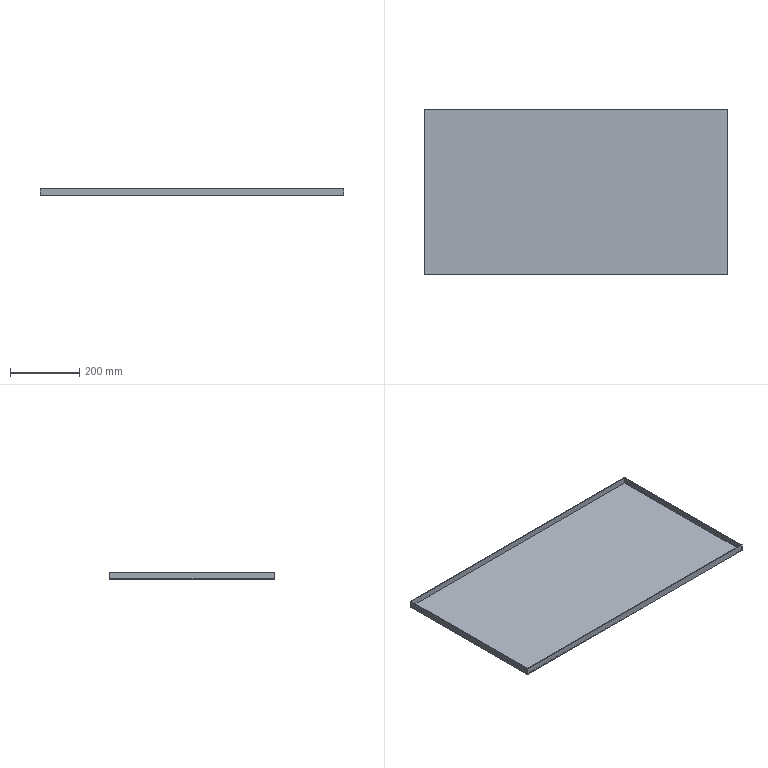Part | STEP file | Sealing plate | 1 solid | 11 faces | box 880 x 480 x 20 mm | volume 942432 mm3 | plane 11
STEP:
#1=CARTESIAN_POINT('',(0.,0.,0.));
#2=DIRECTION('',(0.,0.,1.));
#3=DIRECTION('',(1.,0.,0.));
#4=AXIS2_PLACEMENT_3D('',#1,#2,#3);
#5=CARTESIAN_POINT('',(-440.,-240.,0.));
#6=VERTEX_POINT('',#5);
#7=CARTESIAN_POINT('',(440.,-240.,0.));
#8=VERTEX_POINT('',#7);
#9=CARTESIAN_POINT('',(0.,-240.,0.));
#10=DIRECTION('',(1.,0.,0.));
#11=VECTOR('',#10,1.);
#12=LINE('',#9,#11);
#13=CARTESIAN_POINT('',(0.,0.,0.));
#14=DIRECTION('',(0.,0.,1.));
#15=DIRECTION('',(1.,0.,0.));
#16=AXIS2_PLACEMENT_3D('',#13,#14,#15);
#17=PLANE('',#16);
#18=CARTESIAN_POINT('',(0.,-240.));
#19=DIRECTION('',(1.,0.));
#20=VECTOR('',#19,1.);
#21=LINE('',#18,#20);
#22=(GEOMETRIC_REPRESENTATION_CONTEXT(2)PARAMETRIC_REPRESENTATION_CONTEXT()REPRESENTATION_CONTEXT('',''));
#23=DEFINITIONAL_REPRESENTATION('',(#21),#22);
#24=PCURVE('',#17,#23);
#25=CARTESIAN_POINT('',(-440.,-240.,20.));
#26=DIRECTION('',(0.,1.,0.));
#27=DIRECTION('',(0.,0.,1.));
#28=AXIS2_PLACEMENT_3D('',#25,#26,#27);
#29=PLANE('',#28);
#30=CARTESIAN_POINT('',(-20.,440.));
#31=DIRECTION('',(0.,1.));
#32=VECTOR('',#31,1.);
#33=LINE('',#30,#32);
#34=(GEOMETRIC_REPRESENTATION_CONTEXT(2)PARAMETRIC_REPRESENTATION_CONTEXT()REPRESENTATION_CONTEXT('',''));
#35=DEFINITIONAL_REPRESENTATION('',(#33),#34);
#36=PCURVE('',#29,#35);
#37=SURFACE_CURVE('',#12,(#24,#36),.PCURVE_S1.);
#38=EDGE_CURVE('',#6,#8,#37,.T.);
#39=ORIENTED_EDGE('',*,*,#38,.F.);
#40=CARTESIAN_POINT('',(-440.,240.,0.));
#41=VERTEX_POINT('',#40);
#42=CARTESIAN_POINT('',(-440.,0.,0.));
#43=DIRECTION('',(0.,-1.,0.));
#44=VECTOR('',#43,1.);
#45=LINE('',#42,#44);
#46=CARTESIAN_POINT('',(-440.,0.));
#47=DIRECTION('',(0.,-1.));
#48=VECTOR('',#47,1.);
#49=LINE('',#46,#48);
#50=(GEOMETRIC_REPRESENTATION_CONTEXT(2)PARAMETRIC_REPRESENTATION_CONTEXT()REPRESENTATION_CONTEXT('',''));
#51=DEFINITIONAL_REPRESENTATION('',(#49),#50);
#52=PCURVE('',#17,#51);
#53=CARTESIAN_POINT('',(-440.,240.,20.));
#54=DIRECTION('',(1.,0.,0.));
#55=DIRECTION('',(0.,1.,0.));
#56=AXIS2_PLACEMENT_3D('',#53,#54,#55);
#57=PLANE('',#56);
#58=CARTESIAN_POINT('',(-240.,-20.));
#59=DIRECTION('',(-1.,0.));
#60=VECTOR('',#59,1.);
#61=LINE('',#58,#60);
#62=(GEOMETRIC_REPRESENTATION_CONTEXT(2)PARAMETRIC_REPRESENTATION_CONTEXT()REPRESENTATION_CONTEXT('',''));
#63=DEFINITIONAL_REPRESENTATION('',(#61),#62);
#64=PCURVE('',#57,#63);
#65=SURFACE_CURVE('',#45,(#52,#64),.PCURVE_S1.);
#66=EDGE_CURVE('',#41,#6,#65,.T.);
#67=ORIENTED_EDGE('',*,*,#66,.F.);
#68=CARTESIAN_POINT('',(440.,240.,0.));
#69=VERTEX_POINT('',#68);
#70=CARTESIAN_POINT('',(0.,240.,0.));
#71=DIRECTION('',(-1.,0.,0.));
#72=VECTOR('',#71,1.);
#73=LINE('',#70,#72);
#74=CARTESIAN_POINT('',(0.,240.));
#75=DIRECTION('',(-1.,0.));
#76=VECTOR('',#75,1.);
#77=LINE('',#74,#76);
#78=(GEOMETRIC_REPRESENTATION_CONTEXT(2)PARAMETRIC_REPRESENTATION_CONTEXT()REPRESENTATION_CONTEXT('',''));
#79=DEFINITIONAL_REPRESENTATION('',(#77),#78);
#80=PCURVE('',#17,#79);
#81=CARTESIAN_POINT('',(-440.,240.,20.));
#82=DIRECTION('',(0.,-1.,0.));
#83=DIRECTION('',(0.,0.,-1.));
#84=AXIS2_PLACEMENT_3D('',#81,#82,#83);
#85=PLANE('',#84);
#86=CARTESIAN_POINT('',(20.,440.));
#87=DIRECTION('',(0.,-1.));
#88=VECTOR('',#87,1.);
#89=LINE('',#86,#88);
#90=(GEOMETRIC_REPRESENTATION_CONTEXT(2)PARAMETRIC_REPRESENTATION_CONTEXT()REPRESENTATION_CONTEXT('',''));
#91=DEFINITIONAL_REPRESENTATION('',(#89),#90);
#92=PCURVE('',#85,#91);
#93=SURFACE_CURVE('',#73,(#80,#92),.PCURVE_S1.);
#94=EDGE_CURVE('',#69,#41,#93,.T.);
#95=ORIENTED_EDGE('',*,*,#94,.F.);
#96=CARTESIAN_POINT('',(440.,0.,0.));
#97=DIRECTION('',(0.,1.,0.));
#98=VECTOR('',#97,1.);
#99=LINE('',#96,#98);
#100=CARTESIAN_POINT('',(440.,0.));
#101=DIRECTION('',(0.,1.));
#102=VECTOR('',#101,1.);
#103=LINE('',#100,#102);
#104=(GEOMETRIC_REPRESENTATION_CONTEXT(2)PARAMETRIC_REPRESENTATION_CONTEXT()REPRESENTATION_CONTEXT('',''));
#105=DEFINITIONAL_REPRESENTATION('',(#103),#104);
#106=PCURVE('',#17,#105);
#107=CARTESIAN_POINT('',(440.,240.,20.));
#108=DIRECTION('',(-1.,0.,0.));
#109=DIRECTION('',(0.,-1.,0.));
#110=AXIS2_PLACEMENT_3D('',#107,#108,#109);
#111=PLANE('',#110);
#112=CARTESIAN_POINT('',(240.,-20.));
#113=DIRECTION('',(-1.,0.));
#114=VECTOR('',#113,1.);
#115=LINE('',#112,#114);
#116=(GEOMETRIC_REPRESENTATION_CONTEXT(2)PARAMETRIC_REPRESENTATION_CONTEXT()REPRESENTATION_CONTEXT('',''));
#117=DEFINITIONAL_REPRESENTATION('',(#115),#116);
#118=PCURVE('',#111,#117);
#119=SURFACE_CURVE('',#99,(#106,#118),.PCURVE_S1.);
#120=EDGE_CURVE('',#8,#69,#119,.T.);
#121=ORIENTED_EDGE('',*,*,#120,.F.);
#122=EDGE_LOOP('',(#39,#67,#95,#121));
#123=FACE_BOUND('',#122,.T.);
#124=ADVANCED_FACE('',(#123),#17,.F.);
#125=CARTESIAN_POINT('',(440.,240.,20.));
#126=VERTEX_POINT('',#125);
#127=CARTESIAN_POINT('',(440.,240.,20.));
#128=DIRECTION('',(0.,0.,-1.));
#129=VECTOR('',#128,1.);
#130=LINE('',#127,#129);
#131=CARTESIAN_POINT('',(0.,0.));
#132=DIRECTION('',(0.,-1.));
#133=VECTOR('',#132,1.);
#134=LINE('',#131,#133);
#135=(GEOMETRIC_REPRESENTATION_CONTEXT(2)PARAMETRIC_REPRESENTATION_CONTEXT()REPRESENTATION_CONTEXT('',''));
#136=DEFINITIONAL_REPRESENTATION('',(#134),#135);
#137=PCURVE('',#111,#136);
#138=CARTESIAN_POINT('',(0.,880.));
#139=DIRECTION('',(1.,0.));
#140=VECTOR('',#139,1.);
#141=LINE('',#138,#140);
#142=(GEOMETRIC_REPRESENTATION_CONTEXT(2)PARAMETRIC_REPRESENTATION_CONTEXT()REPRESENTATION_CONTEXT('',''));
#143=DEFINITIONAL_REPRESENTATION('',(#141),#142);
#144=PCURVE('',#85,#143);
#145=SURFACE_CURVE('',#130,(#137,#144),.PCURVE_S1.);
#146=EDGE_CURVE('',#126,#69,#145,.T.);
#147=ORIENTED_EDGE('',*,*,#146,.F.);
#148=CARTESIAN_POINT('',(440.,-240.,20.));
#149=VERTEX_POINT('',#148);
#150=CARTESIAN_POINT('',(440.,240.,20.));
#151=DIRECTION('',(0.,1.,0.));
#152=VECTOR('',#151,1.);
#153=LINE('',#150,#152);
#154=CARTESIAN_POINT('',(0.,0.));
#155=DIRECTION('',(-1.,0.));
#156=VECTOR('',#155,1.);
#157=LINE('',#154,#156);
#158=(GEOMETRIC_REPRESENTATION_CONTEXT(2)PARAMETRIC_REPRESENTATION_CONTEXT()REPRESENTATION_CONTEXT('',''));
#159=DEFINITIONAL_REPRESENTATION('',(#157),#158);
#160=PCURVE('',#111,#159);
#161=CARTESIAN_POINT('',(0.,0.,20.));
#162=DIRECTION('',(0.,0.,1.));
#163=DIRECTION('',(1.,0.,0.));
#164=AXIS2_PLACEMENT_3D('',#161,#162,#163);
#165=PLANE('',#164);
#166=CARTESIAN_POINT('',(440.,240.));
#167=DIRECTION('',(0.,1.));
#168=VECTOR('',#167,1.);
#169=LINE('',#166,#168);
#170=(GEOMETRIC_REPRESENTATION_CONTEXT(2)PARAMETRIC_REPRESENTATION_CONTEXT()REPRESENTATION_CONTEXT('',''));
#171=DEFINITIONAL_REPRESENTATION('',(#169),#170);
#172=PCURVE('',#165,#171);
#173=SURFACE_CURVE('',#153,(#160,#172),.PCURVE_S1.);
#174=EDGE_CURVE('',#149,#126,#173,.T.);
#175=ORIENTED_EDGE('',*,*,#174,.F.);
#176=CARTESIAN_POINT('',(440.,-240.,20.));
#177=DIRECTION('',(0.,0.,1.));
#178=VECTOR('',#177,1.);
#179=LINE('',#176,#178);
#180=CARTESIAN_POINT('',(480.,0.));
#181=DIRECTION('',(0.,1.));
#182=VECTOR('',#181,1.);
#183=LINE('',#180,#182);
#184=(GEOMETRIC_REPRESENTATION_CONTEXT(2)PARAMETRIC_REPRESENTATION_CONTEXT()REPRESENTATION_CONTEXT('',''));
#185=DEFINITIONAL_REPRESENTATION('',(#183),#184);
#186=PCURVE('',#111,#185);
#187=CARTESIAN_POINT('',(0.,880.));
#188=DIRECTION('',(1.,0.));
#189=VECTOR('',#188,1.);
#190=LINE('',#187,#189);
#191=(GEOMETRIC_REPRESENTATION_CONTEXT(2)PARAMETRIC_REPRESENTATION_CONTEXT()REPRESENTATION_CONTEXT('',''));
#192=DEFINITIONAL_REPRESENTATION('',(#190),#191);
#193=PCURVE('',#29,#192);
#194=SURFACE_CURVE('',#179,(#186,#193),.PCURVE_S1.);
#195=EDGE_CURVE('',#8,#149,#194,.T.);
#196=ORIENTED_EDGE('',*,*,#195,.F.);
#197=ORIENTED_EDGE('',*,*,#120,.T.);
#198=EDGE_LOOP('',(#147,#175,#196,#197));
#199=FACE_BOUND('',#198,.T.);
#200=ADVANCED_FACE('',(#199),#111,.F.);
#201=ORIENTED_EDGE('',*,*,#195,.T.);
#202=CARTESIAN_POINT('',(-440.,-240.,20.));
#203=VERTEX_POINT('',#202);
#204=CARTESIAN_POINT('',(-440.,-240.,20.));
#205=DIRECTION('',(1.,0.,0.));
#206=VECTOR('',#205,1.);
#207=LINE('',#204,#206);
#208=CARTESIAN_POINT('',(0.,0.));
#209=DIRECTION('',(0.,1.));
#210=VECTOR('',#209,1.);
#211=LINE('',#208,#210);
#212=(GEOMETRIC_REPRESENTATION_CONTEXT(2)PARAMETRIC_REPRESENTATION_CONTEXT()REPRESENTATION_CONTEXT('',''));
#213=DEFINITIONAL_REPRESENTATION('',(#211),#212);
#214=PCURVE('',#29,#213);
#215=CARTESIAN_POINT('',(-440.,-240.));
#216=DIRECTION('',(1.,0.));
#217=VECTOR('',#216,1.);
#218=LINE('',#215,#217);
#219=(GEOMETRIC_REPRESENTATION_CONTEXT(2)PARAMETRIC_REPRESENTATION_CONTEXT()REPRESENTATION_CONTEXT('',''));
#220=DEFINITIONAL_REPRESENTATION('',(#218),#219);
#221=PCURVE('',#165,#220);
#222=SURFACE_CURVE('',#207,(#214,#221),.PCURVE_S1.);
#223=EDGE_CURVE('',#203,#149,#222,.T.);
#224=ORIENTED_EDGE('',*,*,#223,.F.);
#225=CARTESIAN_POINT('',(-440.,-240.,20.));
#226=DIRECTION('',(0.,0.,1.));
#227=VECTOR('',#226,1.);
#228=LINE('',#225,#227);
#229=CARTESIAN_POINT('',(0.,0.));
#230=DIRECTION('',(1.,0.));
#231=VECTOR('',#230,1.);
#232=LINE('',#229,#231);
#233=(GEOMETRIC_REPRESENTATION_CONTEXT(2)PARAMETRIC_REPRESENTATION_CONTEXT()REPRESENTATION_CONTEXT('',''));
#234=DEFINITIONAL_REPRESENTATION('',(#232),#233);
#235=PCURVE('',#29,#234);
#236=CARTESIAN_POINT('',(-480.,0.));
#237=DIRECTION('',(0.,1.));
#238=VECTOR('',#237,1.);
#239=LINE('',#236,#238);
#240=(GEOMETRIC_REPRESENTATION_CONTEXT(2)PARAMETRIC_REPRESENTATION_CONTEXT()REPRESENTATION_CONTEXT('',''));
#241=DEFINITIONAL_REPRESENTATION('',(#239),#240);
#242=PCURVE('',#57,#241);
#243=SURFACE_CURVE('',#228,(#235,#242),.PCURVE_S1.);
#244=EDGE_CURVE('',#6,#203,#243,.T.);
#245=ORIENTED_EDGE('',*,*,#244,.F.);
#246=ORIENTED_EDGE('',*,*,#38,.T.);
#247=EDGE_LOOP('',(#201,#224,#245,#246));
#248=FACE_BOUND('',#247,.T.);
#249=ADVANCED_FACE('',(#248),#29,.F.);
#250=ORIENTED_EDGE('',*,*,#244,.T.);
#251=CARTESIAN_POINT('',(-440.,240.,20.));
#252=VERTEX_POINT('',#251);
#253=CARTESIAN_POINT('',(-440.,240.,20.));
#254=DIRECTION('',(0.,-1.,0.));
#255=VECTOR('',#254,1.);
#256=LINE('',#253,#255);
#257=CARTESIAN_POINT('',(0.,0.));
#258=DIRECTION('',(-1.,0.));
#259=VECTOR('',#258,1.);
#260=LINE('',#257,#259);
#261=(GEOMETRIC_REPRESENTATION_CONTEXT(2)PARAMETRIC_REPRESENTATION_CONTEXT()REPRESENTATION_CONTEXT('',''));
#262=DEFINITIONAL_REPRESENTATION('',(#260),#261);
#263=PCURVE('',#57,#262);
#264=CARTESIAN_POINT('',(-440.,240.));
#265=DIRECTION('',(0.,-1.));
#266=VECTOR('',#265,1.);
#267=LINE('',#264,#266);
#268=(GEOMETRIC_REPRESENTATION_CONTEXT(2)PARAMETRIC_REPRESENTATION_CONTEXT()REPRESENTATION_CONTEXT('',''));
#269=DEFINITIONAL_REPRESENTATION('',(#267),#268);
#270=PCURVE('',#165,#269);
#271=SURFACE_CURVE('',#256,(#263,#270),.PCURVE_S1.);
#272=EDGE_CURVE('',#252,#203,#271,.T.);
#273=ORIENTED_EDGE('',*,*,#272,.F.);
#274=CARTESIAN_POINT('',(-440.,240.,20.));
#275=DIRECTION('',(0.,0.,1.));
#276=VECTOR('',#275,1.);
#277=LINE('',#274,#276);
#278=CARTESIAN_POINT('',(0.,0.));
#279=DIRECTION('',(0.,1.));
#280=VECTOR('',#279,1.);
#281=LINE('',#278,#280);
#282=(GEOMETRIC_REPRESENTATION_CONTEXT(2)PARAMETRIC_REPRESENTATION_CONTEXT()REPRESENTATION_CONTEXT('',''));
#283=DEFINITIONAL_REPRESENTATION('',(#281),#282);
#284=PCURVE('',#57,#283);
#285=CARTESIAN_POINT('',(0.,0.));
#286=DIRECTION('',(-1.,0.));
#287=VECTOR('',#286,1.);
#288=LINE('',#285,#287);
#289=(GEOMETRIC_REPRESENTATION_CONTEXT(2)PARAMETRIC_REPRESENTATION_CONTEXT()REPRESENTATION_CONTEXT('',''));
#290=DEFINITIONAL_REPRESENTATION('',(#288),#289);
#291=PCURVE('',#85,#290);
#292=SURFACE_CURVE('',#277,(#284,#291),.PCURVE_S1.);
#293=EDGE_CURVE('',#41,#252,#292,.T.);
#294=ORIENTED_EDGE('',*,*,#293,.F.);
#295=ORIENTED_EDGE('',*,*,#66,.T.);
#296=EDGE_LOOP('',(#250,#273,#294,#295));
#297=FACE_BOUND('',#296,.T.);
#298=ADVANCED_FACE('',(#297),#57,.F.);
#299=ORIENTED_EDGE('',*,*,#293,.T.);
#300=CARTESIAN_POINT('',(-440.,240.,20.));
#301=DIRECTION('',(-1.,0.,0.));
#302=VECTOR('',#301,1.);
#303=LINE('',#300,#302);
#304=CARTESIAN_POINT('',(0.,0.));
#305=DIRECTION('',(0.,-1.));
#306=VECTOR('',#305,1.);
#307=LINE('',#304,#306);
#308=(GEOMETRIC_REPRESENTATION_CONTEXT(2)PARAMETRIC_REPRESENTATION_CONTEXT()REPRESENTATION_CONTEXT('',''));
#309=DEFINITIONAL_REPRESENTATION('',(#307),#308);
#310=PCURVE('',#85,#309);
#311=CARTESIAN_POINT('',(-440.,240.));
#312=DIRECTION('',(-1.,0.));
#313=VECTOR('',#312,1.);
#314=LINE('',#311,#313);
#315=(GEOMETRIC_REPRESENTATION_CONTEXT(2)PARAMETRIC_REPRESENTATION_CONTEXT()REPRESENTATION_CONTEXT('',''));
#316=DEFINITIONAL_REPRESENTATION('',(#314),#315);
#317=PCURVE('',#165,#316);
#318=SURFACE_CURVE('',#303,(#310,#317),.PCURVE_S1.);
#319=EDGE_CURVE('',#126,#252,#318,.T.);
#320=ORIENTED_EDGE('',*,*,#319,.F.);
#321=ORIENTED_EDGE('',*,*,#146,.T.);
#322=ORIENTED_EDGE('',*,*,#94,.T.);
#323=EDGE_LOOP('',(#299,#320,#321,#322));
#324=FACE_BOUND('',#323,.T.);
#325=ADVANCED_FACE('',(#324),#85,.F.);
#326=ORIENTED_EDGE('',*,*,#272,.T.);
#327=ORIENTED_EDGE('',*,*,#223,.T.);
#328=ORIENTED_EDGE('',*,*,#174,.T.);
#329=ORIENTED_EDGE('',*,*,#319,.T.);
#330=EDGE_LOOP('',(#326,#327,#328,#329));
#331=FACE_BOUND('',#330,.T.);
#332=CARTESIAN_POINT('',(-438.,-238.,20.));
#333=VERTEX_POINT('',#332);
#334=CARTESIAN_POINT('',(-438.,238.,20.));
#335=VERTEX_POINT('',#334);
#336=CARTESIAN_POINT('',(-438.,0.,20.));
#337=DIRECTION('',(0.,1.,0.));
#338=VECTOR('',#337,1.);
#339=LINE('',#336,#338);
#340=CARTESIAN_POINT('',(-438.,0.));
#341=DIRECTION('',(0.,1.));
#342=VECTOR('',#341,1.);
#343=LINE('',#340,#342);
#344=(GEOMETRIC_REPRESENTATION_CONTEXT(2)PARAMETRIC_REPRESENTATION_CONTEXT()REPRESENTATION_CONTEXT('',''));
#345=DEFINITIONAL_REPRESENTATION('',(#343),#344);
#346=PCURVE('',#165,#345);
#347=CARTESIAN_POINT('',(-438.,240.,20.));
#348=DIRECTION('',(1.,0.,0.));
#349=DIRECTION('',(0.,1.,0.));
#350=AXIS2_PLACEMENT_3D('',#347,#348,#349);
#351=PLANE('',#350);
#352=CARTESIAN_POINT('',(-240.,0.));
#353=DIRECTION('',(1.,0.));
#354=VECTOR('',#353,1.);
#355=LINE('',#352,#354);
#356=(GEOMETRIC_REPRESENTATION_CONTEXT(2)PARAMETRIC_REPRESENTATION_CONTEXT()REPRESENTATION_CONTEXT('',''));
#357=DEFINITIONAL_REPRESENTATION('',(#355),#356);
#358=PCURVE('',#351,#357);
#359=SURFACE_CURVE('',#339,(#346,#358),.PCURVE_S1.);
#360=EDGE_CURVE('',#333,#335,#359,.T.);
#361=ORIENTED_EDGE('',*,*,#360,.T.);
#362=CARTESIAN_POINT('',(438.,238.,20.));
#363=VERTEX_POINT('',#362);
#364=CARTESIAN_POINT('',(0.,238.,20.));
#365=DIRECTION('',(1.,0.,0.));
#366=VECTOR('',#365,1.);
#367=LINE('',#364,#366);
#368=CARTESIAN_POINT('',(0.,238.));
#369=DIRECTION('',(1.,0.));
#370=VECTOR('',#369,1.);
#371=LINE('',#368,#370);
#372=(GEOMETRIC_REPRESENTATION_CONTEXT(2)PARAMETRIC_REPRESENTATION_CONTEXT()REPRESENTATION_CONTEXT('',''));
#373=DEFINITIONAL_REPRESENTATION('',(#371),#372);
#374=PCURVE('',#165,#373);
#375=CARTESIAN_POINT('',(-440.,238.,20.));
#376=DIRECTION('',(0.,-1.,0.));
#377=DIRECTION('',(0.,0.,-1.));
#378=AXIS2_PLACEMENT_3D('',#375,#376,#377);
#379=PLANE('',#378);
#380=CARTESIAN_POINT('',(0.,440.));
#381=DIRECTION('',(0.,1.));
#382=VECTOR('',#381,1.);
#383=LINE('',#380,#382);
#384=(GEOMETRIC_REPRESENTATION_CONTEXT(2)PARAMETRIC_REPRESENTATION_CONTEXT()REPRESENTATION_CONTEXT('',''));
#385=DEFINITIONAL_REPRESENTATION('',(#383),#384);
#386=PCURVE('',#379,#385);
#387=SURFACE_CURVE('',#367,(#374,#386),.PCURVE_S1.);
#388=EDGE_CURVE('',#335,#363,#387,.T.);
#389=ORIENTED_EDGE('',*,*,#388,.T.);
#390=CARTESIAN_POINT('',(438.,-238.,20.));
#391=VERTEX_POINT('',#390);
#392=CARTESIAN_POINT('',(438.,0.,20.));
#393=DIRECTION('',(0.,-1.,0.));
#394=VECTOR('',#393,1.);
#395=LINE('',#392,#394);
#396=CARTESIAN_POINT('',(438.,0.));
#397=DIRECTION('',(0.,-1.));
#398=VECTOR('',#397,1.);
#399=LINE('',#396,#398);
#400=(GEOMETRIC_REPRESENTATION_CONTEXT(2)PARAMETRIC_REPRESENTATION_CONTEXT()REPRESENTATION_CONTEXT('',''));
#401=DEFINITIONAL_REPRESENTATION('',(#399),#400);
#402=PCURVE('',#165,#401);
#403=CARTESIAN_POINT('',(438.,240.,20.));
#404=DIRECTION('',(-1.,0.,0.));
#405=DIRECTION('',(0.,-1.,0.));
#406=AXIS2_PLACEMENT_3D('',#403,#404,#405);
#407=PLANE('',#406);
#408=CARTESIAN_POINT('',(240.,0.));
#409=DIRECTION('',(1.,0.));
#410=VECTOR('',#409,1.);
#411=LINE('',#408,#410);
#412=(GEOMETRIC_REPRESENTATION_CONTEXT(2)PARAMETRIC_REPRESENTATION_CONTEXT()REPRESENTATION_CONTEXT('',''));
#413=DEFINITIONAL_REPRESENTATION('',(#411),#412);
#414=PCURVE('',#407,#413);
#415=SURFACE_CURVE('',#395,(#402,#414),.PCURVE_S1.);
#416=EDGE_CURVE('',#363,#391,#415,.T.);
#417=ORIENTED_EDGE('',*,*,#416,.T.);
#418=CARTESIAN_POINT('',(0.,-238.,20.));
#419=DIRECTION('',(-1.,0.,0.));
#420=VECTOR('',#419,1.);
#421=LINE('',#418,#420);
#422=CARTESIAN_POINT('',(0.,-238.));
#423=DIRECTION('',(-1.,0.));
#424=VECTOR('',#423,1.);
#425=LINE('',#422,#424);
#426=(GEOMETRIC_REPRESENTATION_CONTEXT(2)PARAMETRIC_REPRESENTATION_CONTEXT()REPRESENTATION_CONTEXT('',''));
#427=DEFINITIONAL_REPRESENTATION('',(#425),#426);
#428=PCURVE('',#165,#427);
#429=CARTESIAN_POINT('',(-440.,-238.,20.));
#430=DIRECTION('',(0.,1.,0.));
#431=DIRECTION('',(0.,0.,1.));
#432=AXIS2_PLACEMENT_3D('',#429,#430,#431);
#433=PLANE('',#432);
#434=CARTESIAN_POINT('',(0.,440.));
#435=DIRECTION('',(0.,-1.));
#436=VECTOR('',#435,1.);
#437=LINE('',#434,#436);
#438=(GEOMETRIC_REPRESENTATION_CONTEXT(2)PARAMETRIC_REPRESENTATION_CONTEXT()REPRESENTATION_CONTEXT('',''));
#439=DEFINITIONAL_REPRESENTATION('',(#437),#438);
#440=PCURVE('',#433,#439);
#441=SURFACE_CURVE('',#421,(#428,#440),.PCURVE_S1.);
#442=EDGE_CURVE('',#391,#333,#441,.T.);
#443=ORIENTED_EDGE('',*,*,#442,.T.);
#444=EDGE_LOOP('',(#361,#389,#417,#443));
#445=FACE_BOUND('',#444,.T.);
#446=ADVANCED_FACE('',(#331,#445),#165,.T.);
#447=ORIENTED_EDGE('',*,*,#388,.F.);
#448=CARTESIAN_POINT('',(-438.,238.,2.));
#449=VERTEX_POINT('',#448);
#450=CARTESIAN_POINT('',(-438.,238.,20.));
#451=DIRECTION('',(0.,0.,-1.));
#452=VECTOR('',#451,1.);
#453=LINE('',#450,#452);
#454=CARTESIAN_POINT('',(0.,2.));
#455=DIRECTION('',(1.,0.));
#456=VECTOR('',#455,1.);
#457=LINE('',#454,#456);
#458=(GEOMETRIC_REPRESENTATION_CONTEXT(2)PARAMETRIC_REPRESENTATION_CONTEXT()REPRESENTATION_CONTEXT('',''));
#459=DEFINITIONAL_REPRESENTATION('',(#457),#458);
#460=PCURVE('',#379,#459);
#461=CARTESIAN_POINT('',(-2.,0.));
#462=DIRECTION('',(0.,-1.));
#463=VECTOR('',#462,1.);
#464=LINE('',#461,#463);
#465=(GEOMETRIC_REPRESENTATION_CONTEXT(2)PARAMETRIC_REPRESENTATION_CONTEXT()REPRESENTATION_CONTEXT('',''));
#466=DEFINITIONAL_REPRESENTATION('',(#464),#465);
#467=PCURVE('',#351,#466);
#468=SURFACE_CURVE('',#453,(#460,#467),.PCURVE_S1.);
#469=EDGE_CURVE('',#335,#449,#468,.T.);
#470=ORIENTED_EDGE('',*,*,#469,.T.);
#471=CARTESIAN_POINT('',(438.,238.,2.));
#472=VERTEX_POINT('',#471);
#473=CARTESIAN_POINT('',(-440.,238.,2.));
#474=DIRECTION('',(1.,0.,0.));
#475=VECTOR('',#474,1.);
#476=LINE('',#473,#475);
#477=CARTESIAN_POINT('',(18.,0.));
#478=DIRECTION('',(0.,1.));
#479=VECTOR('',#478,1.);
#480=LINE('',#477,#479);
#481=(GEOMETRIC_REPRESENTATION_CONTEXT(2)PARAMETRIC_REPRESENTATION_CONTEXT()REPRESENTATION_CONTEXT('',''));
#482=DEFINITIONAL_REPRESENTATION('',(#480),#481);
#483=PCURVE('',#379,#482);
#484=CARTESIAN_POINT('',(0.,0.,2.));
#485=DIRECTION('',(0.,0.,1.));
#486=DIRECTION('',(1.,0.,0.));
#487=AXIS2_PLACEMENT_3D('',#484,#485,#486);
#488=PLANE('',#487);
#489=CARTESIAN_POINT('',(-440.,238.));
#490=DIRECTION('',(1.,0.));
#491=VECTOR('',#490,1.);
#492=LINE('',#489,#491);
#493=(GEOMETRIC_REPRESENTATION_CONTEXT(2)PARAMETRIC_REPRESENTATION_CONTEXT()REPRESENTATION_CONTEXT('',''));
#494=DEFINITIONAL_REPRESENTATION('',(#492),#493);
#495=PCURVE('',#488,#494);
#496=SURFACE_CURVE('',#476,(#483,#495),.PCURVE_S1.);
#497=EDGE_CURVE('',#449,#472,#496,.T.);
#498=ORIENTED_EDGE('',*,*,#497,.T.);
#499=CARTESIAN_POINT('',(438.,238.,20.));
#500=DIRECTION('',(0.,0.,1.));
#501=VECTOR('',#500,1.);
#502=LINE('',#499,#501);
#503=CARTESIAN_POINT('',(0.,878.));
#504=DIRECTION('',(-1.,0.));
#505=VECTOR('',#504,1.);
#506=LINE('',#503,#505);
#507=(GEOMETRIC_REPRESENTATION_CONTEXT(2)PARAMETRIC_REPRESENTATION_CONTEXT()REPRESENTATION_CONTEXT('',''));
#508=DEFINITIONAL_REPRESENTATION('',(#506),#507);
#509=PCURVE('',#379,#508);
#510=CARTESIAN_POINT('',(2.,0.));
#511=DIRECTION('',(0.,1.));
#512=VECTOR('',#511,1.);
#513=LINE('',#510,#512);
#514=(GEOMETRIC_REPRESENTATION_CONTEXT(2)PARAMETRIC_REPRESENTATION_CONTEXT()REPRESENTATION_CONTEXT('',''));
#515=DEFINITIONAL_REPRESENTATION('',(#513),#514);
#516=PCURVE('',#407,#515);
#517=SURFACE_CURVE('',#502,(#509,#516),.PCURVE_S1.);
#518=EDGE_CURVE('',#472,#363,#517,.T.);
#519=ORIENTED_EDGE('',*,*,#518,.T.);
#520=EDGE_LOOP('',(#447,#470,#498,#519));
#521=FACE_BOUND('',#520,.T.);
#522=ADVANCED_FACE('',(#521),#379,.T.);
#523=ORIENTED_EDGE('',*,*,#360,.F.);
#524=CARTESIAN_POINT('',(-438.,-238.,2.));
#525=VERTEX_POINT('',#524);
#526=CARTESIAN_POINT('',(-438.,-238.,20.));
#527=DIRECTION('',(0.,0.,-1.));
#528=VECTOR('',#527,1.);
#529=LINE('',#526,#528);
#530=CARTESIAN_POINT('',(-478.,0.));
#531=DIRECTION('',(0.,-1.));
#532=VECTOR('',#531,1.);
#533=LINE('',#530,#532);
#534=(GEOMETRIC_REPRESENTATION_CONTEXT(2)PARAMETRIC_REPRESENTATION_CONTEXT()REPRESENTATION_CONTEXT('',''));
#535=DEFINITIONAL_REPRESENTATION('',(#533),#534);
#536=PCURVE('',#351,#535);
#537=CARTESIAN_POINT('',(0.,2.));
#538=DIRECTION('',(-1.,0.));
#539=VECTOR('',#538,1.);
#540=LINE('',#537,#539);
#541=(GEOMETRIC_REPRESENTATION_CONTEXT(2)PARAMETRIC_REPRESENTATION_CONTEXT()REPRESENTATION_CONTEXT('',''));
#542=DEFINITIONAL_REPRESENTATION('',(#540),#541);
#543=PCURVE('',#433,#542);
#544=SURFACE_CURVE('',#529,(#536,#543),.PCURVE_S1.);
#545=EDGE_CURVE('',#333,#525,#544,.T.);
#546=ORIENTED_EDGE('',*,*,#545,.T.);
#547=CARTESIAN_POINT('',(-438.,240.,2.));
#548=DIRECTION('',(0.,1.,0.));
#549=VECTOR('',#548,1.);
#550=LINE('',#547,#549);
#551=CARTESIAN_POINT('',(0.,-18.));
#552=DIRECTION('',(1.,0.));
#553=VECTOR('',#552,1.);
#554=LINE('',#551,#553);
#555=(GEOMETRIC_REPRESENTATION_CONTEXT(2)PARAMETRIC_REPRESENTATION_CONTEXT()REPRESENTATION_CONTEXT('',''));
#556=DEFINITIONAL_REPRESENTATION('',(#554),#555);
#557=PCURVE('',#351,#556);
#558=CARTESIAN_POINT('',(-438.,240.));
#559=DIRECTION('',(0.,1.));
#560=VECTOR('',#559,1.);
#561=LINE('',#558,#560);
#562=(GEOMETRIC_REPRESENTATION_CONTEXT(2)PARAMETRIC_REPRESENTATION_CONTEXT()REPRESENTATION_CONTEXT('',''));
#563=DEFINITIONAL_REPRESENTATION('',(#561),#562);
#564=PCURVE('',#488,#563);
#565=SURFACE_CURVE('',#550,(#557,#564),.PCURVE_S1.);
#566=EDGE_CURVE('',#525,#449,#565,.T.);
#567=ORIENTED_EDGE('',*,*,#566,.T.);
#568=ORIENTED_EDGE('',*,*,#469,.F.);
#569=EDGE_LOOP('',(#523,#546,#567,#568));
#570=FACE_BOUND('',#569,.T.);
#571=ADVANCED_FACE('',(#570),#351,.T.);
#572=ORIENTED_EDGE('',*,*,#442,.F.);
#573=CARTESIAN_POINT('',(438.,-238.,2.));
#574=VERTEX_POINT('',#573);
#575=CARTESIAN_POINT('',(438.,-238.,20.));
#576=DIRECTION('',(0.,0.,-1.));
#577=VECTOR('',#576,1.);
#578=LINE('',#575,#577);
#579=CARTESIAN_POINT('',(0.,878.));
#580=DIRECTION('',(-1.,0.));
#581=VECTOR('',#580,1.);
#582=LINE('',#579,#581);
#583=(GEOMETRIC_REPRESENTATION_CONTEXT(2)PARAMETRIC_REPRESENTATION_CONTEXT()REPRESENTATION_CONTEXT('',''));
#584=DEFINITIONAL_REPRESENTATION('',(#582),#583);
#585=PCURVE('',#433,#584);
#586=CARTESIAN_POINT('',(478.,0.));
#587=DIRECTION('',(0.,-1.));
#588=VECTOR('',#587,1.);
#589=LINE('',#586,#588);
#590=(GEOMETRIC_REPRESENTATION_CONTEXT(2)PARAMETRIC_REPRESENTATION_CONTEXT()REPRESENTATION_CONTEXT('',''));
#591=DEFINITIONAL_REPRESENTATION('',(#589),#590);
#592=PCURVE('',#407,#591);
#593=SURFACE_CURVE('',#578,(#585,#592),.PCURVE_S1.);
#594=EDGE_CURVE('',#391,#574,#593,.T.);
#595=ORIENTED_EDGE('',*,*,#594,.T.);
#596=CARTESIAN_POINT('',(-440.,-238.,2.));
#597=DIRECTION('',(-1.,0.,0.));
#598=VECTOR('',#597,1.);
#599=LINE('',#596,#598);
#600=CARTESIAN_POINT('',(-18.,0.));
#601=DIRECTION('',(0.,-1.));
#602=VECTOR('',#601,1.);
#603=LINE('',#600,#602);
#604=(GEOMETRIC_REPRESENTATION_CONTEXT(2)PARAMETRIC_REPRESENTATION_CONTEXT()REPRESENTATION_CONTEXT('',''));
#605=DEFINITIONAL_REPRESENTATION('',(#603),#604);
#606=PCURVE('',#433,#605);
#607=CARTESIAN_POINT('',(-440.,-238.));
#608=DIRECTION('',(-1.,0.));
#609=VECTOR('',#608,1.);
#610=LINE('',#607,#609);
#611=(GEOMETRIC_REPRESENTATION_CONTEXT(2)PARAMETRIC_REPRESENTATION_CONTEXT()REPRESENTATION_CONTEXT('',''));
#612=DEFINITIONAL_REPRESENTATION('',(#610),#611);
#613=PCURVE('',#488,#612);
#614=SURFACE_CURVE('',#599,(#606,#613),.PCURVE_S1.);
#615=EDGE_CURVE('',#574,#525,#614,.T.);
#616=ORIENTED_EDGE('',*,*,#615,.T.);
#617=ORIENTED_EDGE('',*,*,#545,.F.);
#618=EDGE_LOOP('',(#572,#595,#616,#617));
#619=FACE_BOUND('',#618,.T.);
#620=ADVANCED_FACE('',(#619),#433,.T.);
#621=ORIENTED_EDGE('',*,*,#416,.F.);
#622=ORIENTED_EDGE('',*,*,#518,.F.);
#623=CARTESIAN_POINT('',(438.,240.,2.));
#624=DIRECTION('',(0.,-1.,0.));
#625=VECTOR('',#624,1.);
#626=LINE('',#623,#625);
#627=CARTESIAN_POINT('',(0.,-18.));
#628=DIRECTION('',(1.,0.));
#629=VECTOR('',#628,1.);
#630=LINE('',#627,#629);
#631=(GEOMETRIC_REPRESENTATION_CONTEXT(2)PARAMETRIC_REPRESENTATION_CONTEXT()REPRESENTATION_CONTEXT('',''));
#632=DEFINITIONAL_REPRESENTATION('',(#630),#631);
#633=PCURVE('',#407,#632);
#634=CARTESIAN_POINT('',(438.,240.));
#635=DIRECTION('',(0.,-1.));
#636=VECTOR('',#635,1.);
#637=LINE('',#634,#636);
#638=(GEOMETRIC_REPRESENTATION_CONTEXT(2)PARAMETRIC_REPRESENTATION_CONTEXT()REPRESENTATION_CONTEXT('',''));
#639=DEFINITIONAL_REPRESENTATION('',(#637),#638);
#640=PCURVE('',#488,#639);
#641=SURFACE_CURVE('',#626,(#633,#640),.PCURVE_S1.);
#642=EDGE_CURVE('',#472,#574,#641,.T.);
#643=ORIENTED_EDGE('',*,*,#642,.T.);
#644=ORIENTED_EDGE('',*,*,#594,.F.);
#645=EDGE_LOOP('',(#621,#622,#643,#644));
#646=FACE_BOUND('',#645,.T.);
#647=ADVANCED_FACE('',(#646),#407,.T.);
#648=ORIENTED_EDGE('',*,*,#566,.F.);
#649=ORIENTED_EDGE('',*,*,#615,.F.);
#650=ORIENTED_EDGE('',*,*,#642,.F.);
#651=ORIENTED_EDGE('',*,*,#497,.F.);
#652=EDGE_LOOP('',(#648,#649,#650,#651));
#653=FACE_BOUND('',#652,.T.);
#654=ADVANCED_FACE('',(#653),#488,.T.);
#655=CLOSED_SHELL('',(#124,#200,#249,#298,#325,#446,#522,#571,#620,#647,#654));
#656=MANIFOLD_SOLID_BREP('',#655);
#657=(LENGTH_UNIT()NAMED_UNIT(*)SI_UNIT(.MILLI.,.METRE.));
#658=UNCERTAINTY_MEASURE_WITH_UNIT(LENGTH_MEASURE(0.0000001),#657,'','');
#659=(NAMED_UNIT(*)PLANE_ANGLE_UNIT()SI_UNIT($,.RADIAN.));
#660=(NAMED_UNIT(*)SI_UNIT($,.STERADIAN.)SOLID_ANGLE_UNIT());
#661=(GEOMETRIC_REPRESENTATION_CONTEXT(3)GLOBAL_UNCERTAINTY_ASSIGNED_CONTEXT((#658))GLOBAL_UNIT_ASSIGNED_CONTEXT((#657,#659,#660))REPRESENTATION_CONTEXT('',''));
#662=ADVANCED_BREP_SHAPE_REPRESENTATION('',(#4,#656),#661);